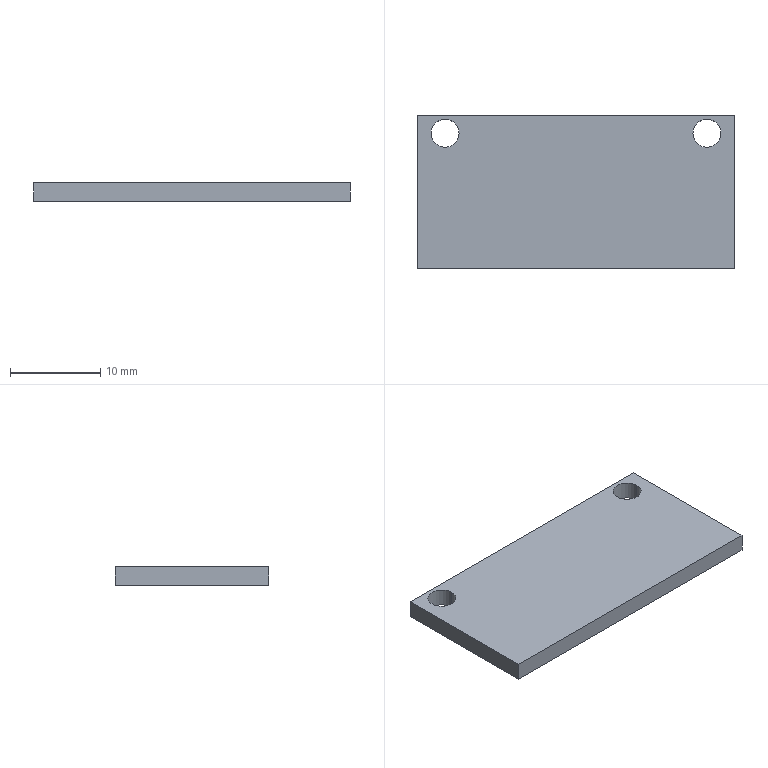Part | STEP file | 02-18 press plate | 1 solid | 10 faces | box 35 x 17 x 2 mm | volume 1160 mm3 | plane 6 | cylinder 4 | commonest cylinder face diameters 3.1 x4
STEP:
#1=CARTESIAN_POINT('',(12.95,6.5,0.));
#2=VERTEX_POINT('',#1);
#3=CARTESIAN_POINT('',(16.05,6.5,0.));
#4=VERTEX_POINT('',#3);
#5=CARTESIAN_POINT('',(14.5,6.5,0.));
#6=DIRECTION('',(0.,0.,1.));
#7=DIRECTION('',(1.,0.,0.));
#8=AXIS2_PLACEMENT_3D('',#5,#6,#7);
#9=CIRCLE('',#8,1.55);
#10=EDGE_CURVE('',#2,#4,#9,.T.);
#11=ORIENTED_EDGE('',*,*,#10,.F.);
#12=CARTESIAN_POINT('',(12.95,6.5,2.));
#13=VERTEX_POINT('',#12);
#14=CARTESIAN_POINT('',(12.95,6.5,2.));
#15=DIRECTION('',(0.,0.,1.));
#16=VECTOR('',#15,1000.);
#17=LINE('',#14,#16);
#18=EDGE_CURVE('',#2,#13,#17,.T.);
#19=ORIENTED_EDGE('',*,*,#18,.T.);
#20=CARTESIAN_POINT('',(16.05,6.5,2.));
#21=VERTEX_POINT('',#20);
#22=CARTESIAN_POINT('',(14.5,6.5,2.));
#23=DIRECTION('',(0.,0.,1.));
#24=DIRECTION('',(1.,0.,0.));
#25=AXIS2_PLACEMENT_3D('',#22,#23,#24);
#26=CIRCLE('',#25,1.55);
#27=EDGE_CURVE('',#13,#21,#26,.T.);
#28=ORIENTED_EDGE('',*,*,#27,.T.);
#29=CARTESIAN_POINT('',(16.05,6.5,2.));
#30=DIRECTION('',(0.,0.,1.));
#31=VECTOR('',#30,1000.);
#32=LINE('',#29,#31);
#33=EDGE_CURVE('',#4,#21,#32,.T.);
#34=ORIENTED_EDGE('',*,*,#33,.F.);
#35=EDGE_LOOP('',(#11,#19,#28,#34));
#36=FACE_OUTER_BOUND('',#35,.T.);
#37=CARTESIAN_POINT('',(14.5,6.5,2.));
#38=DIRECTION('',(0.,0.,1.));
#39=DIRECTION('',(1.,0.,0.));
#40=AXIS2_PLACEMENT_3D('',#37,#38,#39);
#41=CYLINDRICAL_SURFACE('',#40,1.55);
#42=ADVANCED_FACE('',(#36),#41,.F.);
#43=CARTESIAN_POINT('',(-16.05,6.5,0.));
#44=VERTEX_POINT('',#43);
#45=CARTESIAN_POINT('',(-12.95,6.5,0.));
#46=VERTEX_POINT('',#45);
#47=CARTESIAN_POINT('',(-14.5,6.5,0.));
#48=DIRECTION('',(0.,0.,1.));
#49=DIRECTION('',(1.,0.,0.));
#50=AXIS2_PLACEMENT_3D('',#47,#48,#49);
#51=CIRCLE('',#50,1.55);
#52=EDGE_CURVE('',#44,#46,#51,.T.);
#53=ORIENTED_EDGE('',*,*,#52,.F.);
#54=CARTESIAN_POINT('',(-16.05,6.5,2.));
#55=VERTEX_POINT('',#54);
#56=CARTESIAN_POINT('',(-16.05,6.5,2.));
#57=DIRECTION('',(0.,0.,1.));
#58=VECTOR('',#57,1000.);
#59=LINE('',#56,#58);
#60=EDGE_CURVE('',#44,#55,#59,.T.);
#61=ORIENTED_EDGE('',*,*,#60,.T.);
#62=CARTESIAN_POINT('',(-12.95,6.5,2.));
#63=VERTEX_POINT('',#62);
#64=CARTESIAN_POINT('',(-14.5,6.5,2.));
#65=DIRECTION('',(0.,0.,1.));
#66=DIRECTION('',(1.,0.,0.));
#67=AXIS2_PLACEMENT_3D('',#64,#65,#66);
#68=CIRCLE('',#67,1.55);
#69=EDGE_CURVE('',#55,#63,#68,.T.);
#70=ORIENTED_EDGE('',*,*,#69,.T.);
#71=CARTESIAN_POINT('',(-12.95,6.5,2.));
#72=DIRECTION('',(0.,0.,1.));
#73=VECTOR('',#72,1000.);
#74=LINE('',#71,#73);
#75=EDGE_CURVE('',#46,#63,#74,.T.);
#76=ORIENTED_EDGE('',*,*,#75,.F.);
#77=EDGE_LOOP('',(#53,#61,#70,#76));
#78=FACE_OUTER_BOUND('',#77,.T.);
#79=CARTESIAN_POINT('',(-14.5,6.5,2.));
#80=DIRECTION('',(0.,0.,1.));
#81=DIRECTION('',(1.,0.,0.));
#82=AXIS2_PLACEMENT_3D('',#79,#80,#81);
#83=CYLINDRICAL_SURFACE('',#82,1.55);
#84=ADVANCED_FACE('',(#78),#83,.F.);
#85=CARTESIAN_POINT('',(-17.5,8.5,0.));
#86=VERTEX_POINT('',#85);
#87=CARTESIAN_POINT('',(-17.5,-8.5,0.));
#88=VERTEX_POINT('',#87);
#89=CARTESIAN_POINT('',(-17.5,-8.5,0.));
#90=DIRECTION('',(0.,-1.,0.));
#91=VECTOR('',#90,1000.);
#92=LINE('',#89,#91);
#93=EDGE_CURVE('',#86,#88,#92,.T.);
#94=ORIENTED_EDGE('',*,*,#93,.T.);
#95=CARTESIAN_POINT('',(-17.5,-8.5,2.));
#96=VERTEX_POINT('',#95);
#97=CARTESIAN_POINT('',(-17.5,-8.5,2.));
#98=DIRECTION('',(0.,0.,-1.));
#99=VECTOR('',#98,1000.);
#100=LINE('',#97,#99);
#101=EDGE_CURVE('',#96,#88,#100,.T.);
#102=ORIENTED_EDGE('',*,*,#101,.F.);
#103=CARTESIAN_POINT('',(-17.5,8.5,2.));
#104=VERTEX_POINT('',#103);
#105=CARTESIAN_POINT('',(-17.5,-8.5,2.));
#106=DIRECTION('',(0.,-1.,0.));
#107=VECTOR('',#106,1000.);
#108=LINE('',#105,#107);
#109=EDGE_CURVE('',#104,#96,#108,.T.);
#110=ORIENTED_EDGE('',*,*,#109,.F.);
#111=CARTESIAN_POINT('',(-17.5,8.5,2.));
#112=DIRECTION('',(0.,0.,-1.));
#113=VECTOR('',#112,1000.);
#114=LINE('',#111,#113);
#115=EDGE_CURVE('',#104,#86,#114,.T.);
#116=ORIENTED_EDGE('',*,*,#115,.T.);
#117=EDGE_LOOP('',(#94,#102,#110,#116));
#118=FACE_OUTER_BOUND('',#117,.T.);
#119=CARTESIAN_POINT('',(-17.5,-8.5,2.));
#120=DIRECTION('',(1.,0.,0.));
#121=DIRECTION('',(0.,0.,-1.));
#122=AXIS2_PLACEMENT_3D('',#119,#120,#121);
#123=PLANE('',#122);
#124=ADVANCED_FACE('',(#118),#123,.F.);
#125=CARTESIAN_POINT('',(17.5,-8.5,0.));
#126=VERTEX_POINT('',#125);
#127=CARTESIAN_POINT('',(17.5,-8.5,0.));
#128=DIRECTION('',(1.,0.,0.));
#129=VECTOR('',#128,1000.);
#130=LINE('',#127,#129);
#131=EDGE_CURVE('',#88,#126,#130,.T.);
#132=ORIENTED_EDGE('',*,*,#131,.T.);
#133=CARTESIAN_POINT('',(17.5,-8.5,2.));
#134=VERTEX_POINT('',#133);
#135=CARTESIAN_POINT('',(17.5,-8.5,2.));
#136=DIRECTION('',(0.,0.,-1.));
#137=VECTOR('',#136,1000.);
#138=LINE('',#135,#137);
#139=EDGE_CURVE('',#134,#126,#138,.T.);
#140=ORIENTED_EDGE('',*,*,#139,.F.);
#141=CARTESIAN_POINT('',(17.5,-8.5,2.));
#142=DIRECTION('',(1.,0.,0.));
#143=VECTOR('',#142,1000.);
#144=LINE('',#141,#143);
#145=EDGE_CURVE('',#96,#134,#144,.T.);
#146=ORIENTED_EDGE('',*,*,#145,.F.);
#147=ORIENTED_EDGE('',*,*,#101,.T.);
#148=EDGE_LOOP('',(#132,#140,#146,#147));
#149=FACE_OUTER_BOUND('',#148,.T.);
#150=CARTESIAN_POINT('',(17.5,-8.5,2.));
#151=DIRECTION('',(0.,1.,0.));
#152=DIRECTION('',(-1.,0.,0.));
#153=AXIS2_PLACEMENT_3D('',#150,#151,#152);
#154=PLANE('',#153);
#155=ADVANCED_FACE('',(#149),#154,.F.);
#156=CARTESIAN_POINT('',(17.5,8.5,0.));
#157=VERTEX_POINT('',#156);
#158=CARTESIAN_POINT('',(17.5,-8.5,0.));
#159=DIRECTION('',(0.,1.,0.));
#160=VECTOR('',#159,1000.);
#161=LINE('',#158,#160);
#162=EDGE_CURVE('',#126,#157,#161,.T.);
#163=ORIENTED_EDGE('',*,*,#162,.T.);
#164=CARTESIAN_POINT('',(17.5,8.5,2.));
#165=VERTEX_POINT('',#164);
#166=CARTESIAN_POINT('',(17.5,8.5,2.));
#167=DIRECTION('',(0.,0.,-1.));
#168=VECTOR('',#167,1000.);
#169=LINE('',#166,#168);
#170=EDGE_CURVE('',#165,#157,#169,.T.);
#171=ORIENTED_EDGE('',*,*,#170,.F.);
#172=CARTESIAN_POINT('',(17.5,-8.5,2.));
#173=DIRECTION('',(0.,1.,0.));
#174=VECTOR('',#173,1000.);
#175=LINE('',#172,#174);
#176=EDGE_CURVE('',#134,#165,#175,.T.);
#177=ORIENTED_EDGE('',*,*,#176,.F.);
#178=ORIENTED_EDGE('',*,*,#139,.T.);
#179=EDGE_LOOP('',(#163,#171,#177,#178));
#180=FACE_OUTER_BOUND('',#179,.T.);
#181=CARTESIAN_POINT('',(17.5,-8.5,2.));
#182=DIRECTION('',(-1.,0.,0.));
#183=DIRECTION('',(0.,0.,1.));
#184=AXIS2_PLACEMENT_3D('',#181,#182,#183);
#185=PLANE('',#184);
#186=ADVANCED_FACE('',(#180),#185,.F.);
#187=CARTESIAN_POINT('',(17.5,8.5,0.));
#188=DIRECTION('',(-1.,0.,0.));
#189=VECTOR('',#188,1000.);
#190=LINE('',#187,#189);
#191=EDGE_CURVE('',#157,#86,#190,.T.);
#192=ORIENTED_EDGE('',*,*,#191,.T.);
#193=ORIENTED_EDGE('',*,*,#115,.F.);
#194=CARTESIAN_POINT('',(17.5,8.5,2.));
#195=DIRECTION('',(-1.,0.,0.));
#196=VECTOR('',#195,1000.);
#197=LINE('',#194,#196);
#198=EDGE_CURVE('',#165,#104,#197,.T.);
#199=ORIENTED_EDGE('',*,*,#198,.F.);
#200=ORIENTED_EDGE('',*,*,#170,.T.);
#201=EDGE_LOOP('',(#192,#193,#199,#200));
#202=FACE_OUTER_BOUND('',#201,.T.);
#203=CARTESIAN_POINT('',(17.5,8.5,2.));
#204=DIRECTION('',(0.,-1.,0.));
#205=DIRECTION('',(1.,0.,0.));
#206=AXIS2_PLACEMENT_3D('',#203,#204,#205);
#207=PLANE('',#206);
#208=ADVANCED_FACE('',(#202),#207,.F.);
#209=CARTESIAN_POINT('',(14.5,6.5,2.));
#210=DIRECTION('',(0.,0.,1.));
#211=DIRECTION('',(1.,0.,0.));
#212=AXIS2_PLACEMENT_3D('',#209,#210,#211);
#213=CIRCLE('',#212,1.55);
#214=EDGE_CURVE('',#21,#13,#213,.T.);
#215=ORIENTED_EDGE('',*,*,#214,.F.);
#216=ORIENTED_EDGE('',*,*,#27,.F.);
#217=EDGE_LOOP('',(#215,#216));
#218=FACE_BOUND('',#217,.T.);
#219=CARTESIAN_POINT('',(-14.5,6.5,2.));
#220=DIRECTION('',(0.,0.,1.));
#221=DIRECTION('',(1.,0.,0.));
#222=AXIS2_PLACEMENT_3D('',#219,#220,#221);
#223=CIRCLE('',#222,1.55);
#224=EDGE_CURVE('',#63,#55,#223,.T.);
#225=ORIENTED_EDGE('',*,*,#224,.F.);
#226=ORIENTED_EDGE('',*,*,#69,.F.);
#227=EDGE_LOOP('',(#225,#226));
#228=FACE_BOUND('',#227,.T.);
#229=ORIENTED_EDGE('',*,*,#109,.T.);
#230=ORIENTED_EDGE('',*,*,#145,.T.);
#231=ORIENTED_EDGE('',*,*,#176,.T.);
#232=ORIENTED_EDGE('',*,*,#198,.T.);
#233=EDGE_LOOP('',(#229,#230,#231,#232));
#234=FACE_OUTER_BOUND('',#233,.T.);
#235=CARTESIAN_POINT('',(-17.5,8.5,2.));
#236=DIRECTION('',(0.,0.,1.));
#237=DIRECTION('',(1.,0.,0.));
#238=AXIS2_PLACEMENT_3D('',#235,#236,#237);
#239=PLANE('',#238);
#240=ADVANCED_FACE('',(#218,#228,#234),#239,.T.);
#241=CARTESIAN_POINT('',(14.5,6.5,0.));
#242=DIRECTION('',(0.,0.,1.));
#243=DIRECTION('',(1.,0.,0.));
#244=AXIS2_PLACEMENT_3D('',#241,#242,#243);
#245=CIRCLE('',#244,1.55);
#246=EDGE_CURVE('',#4,#2,#245,.T.);
#247=ORIENTED_EDGE('',*,*,#246,.T.);
#248=ORIENTED_EDGE('',*,*,#10,.T.);
#249=EDGE_LOOP('',(#247,#248));
#250=FACE_BOUND('',#249,.T.);
#251=CARTESIAN_POINT('',(-14.5,6.5,0.));
#252=DIRECTION('',(0.,0.,1.));
#253=DIRECTION('',(1.,0.,0.));
#254=AXIS2_PLACEMENT_3D('',#251,#252,#253);
#255=CIRCLE('',#254,1.55);
#256=EDGE_CURVE('',#46,#44,#255,.T.);
#257=ORIENTED_EDGE('',*,*,#256,.T.);
#258=ORIENTED_EDGE('',*,*,#52,.T.);
#259=EDGE_LOOP('',(#257,#258));
#260=FACE_BOUND('',#259,.T.);
#261=ORIENTED_EDGE('',*,*,#93,.F.);
#262=ORIENTED_EDGE('',*,*,#191,.F.);
#263=ORIENTED_EDGE('',*,*,#162,.F.);
#264=ORIENTED_EDGE('',*,*,#131,.F.);
#265=EDGE_LOOP('',(#261,#262,#263,#264));
#266=FACE_OUTER_BOUND('',#265,.T.);
#267=CARTESIAN_POINT('',(-17.5,8.5,0.));
#268=DIRECTION('',(0.,0.,1.));
#269=DIRECTION('',(1.,0.,0.));
#270=AXIS2_PLACEMENT_3D('',#267,#268,#269);
#271=PLANE('',#270);
#272=ADVANCED_FACE('',(#250,#260,#266),#271,.F.);
#273=ORIENTED_EDGE('',*,*,#60,.F.);
#274=ORIENTED_EDGE('',*,*,#256,.F.);
#275=ORIENTED_EDGE('',*,*,#75,.T.);
#276=ORIENTED_EDGE('',*,*,#224,.T.);
#277=EDGE_LOOP('',(#273,#274,#275,#276));
#278=FACE_OUTER_BOUND('',#277,.T.);
#279=CARTESIAN_POINT('',(-14.5,6.5,2.));
#280=DIRECTION('',(0.,0.,1.));
#281=DIRECTION('',(1.,0.,0.));
#282=AXIS2_PLACEMENT_3D('',#279,#280,#281);
#283=CYLINDRICAL_SURFACE('',#282,1.55);
#284=ADVANCED_FACE('',(#278),#283,.F.);
#285=ORIENTED_EDGE('',*,*,#18,.F.);
#286=ORIENTED_EDGE('',*,*,#246,.F.);
#287=ORIENTED_EDGE('',*,*,#33,.T.);
#288=ORIENTED_EDGE('',*,*,#214,.T.);
#289=EDGE_LOOP('',(#285,#286,#287,#288));
#290=FACE_OUTER_BOUND('',#289,.T.);
#291=CARTESIAN_POINT('',(14.5,6.5,2.));
#292=DIRECTION('',(0.,0.,1.));
#293=DIRECTION('',(1.,0.,0.));
#294=AXIS2_PLACEMENT_3D('',#291,#292,#293);
#295=CYLINDRICAL_SURFACE('',#294,1.55);
#296=ADVANCED_FACE('',(#290),#295,.F.);
#297=CLOSED_SHELL('',(#42,#84,#124,#155,#186,#208,#240,#272,#284,#296));
#298=MANIFOLD_SOLID_BREP('',#297);
#299=CARTESIAN_POINT('',(0.,0.,0.));
#300=DIRECTION('',(0.,0.,1.));
#301=DIRECTION('',(1.,0.,0.));
#302=AXIS2_PLACEMENT_3D('',#299,#300,#301);
#303=(LENGTH_UNIT()NAMED_UNIT(*)SI_UNIT(.MILLI.,.METRE.));
#304=UNCERTAINTY_MEASURE_WITH_UNIT(LENGTH_MEASURE(0.00001),#303,'','');
#305=(NAMED_UNIT(*)PLANE_ANGLE_UNIT()SI_UNIT($,.RADIAN.));
#306=(NAMED_UNIT(*)SI_UNIT($,.STERADIAN.)SOLID_ANGLE_UNIT());
#307=(GEOMETRIC_REPRESENTATION_CONTEXT(3)GLOBAL_UNCERTAINTY_ASSIGNED_CONTEXT((#304))GLOBAL_UNIT_ASSIGNED_CONTEXT((#303,#305,#306))REPRESENTATION_CONTEXT('',''));
#308=ADVANCED_BREP_SHAPE_REPRESENTATION('',(#298,#302),#307);